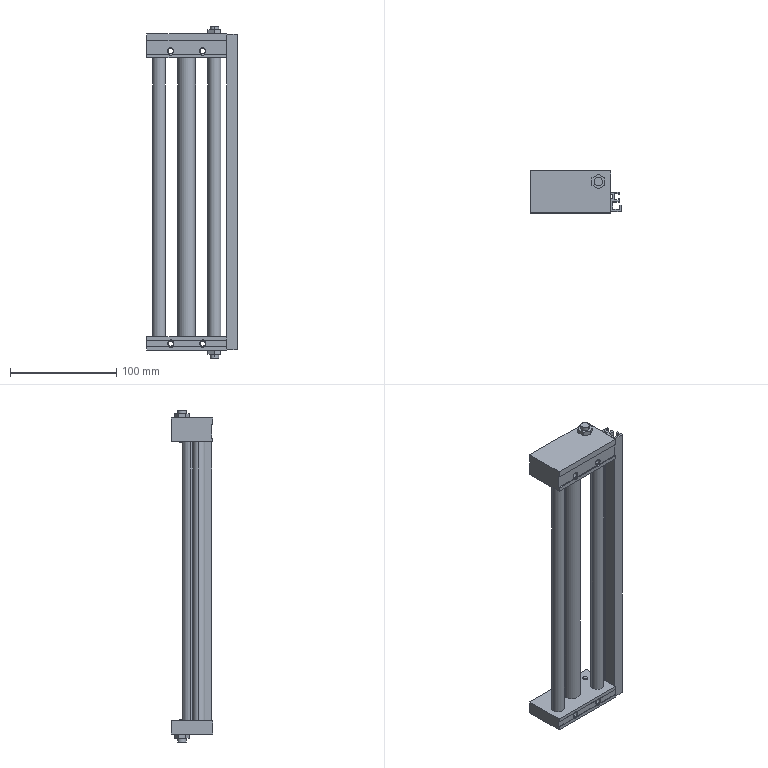Part | STEP file | Mount electronic clip rodless cylinder 1-2-1 | 1 solid | 146 faces | box 85 x 39 x 312 mm | volume 237778 mm3 | plane 78 | cylinder 42 | cone 26 | commonest cylinder face diameters 4.92 x8 5.6 x8 9.5 x8 4 x4 4.13 x4 8 x4